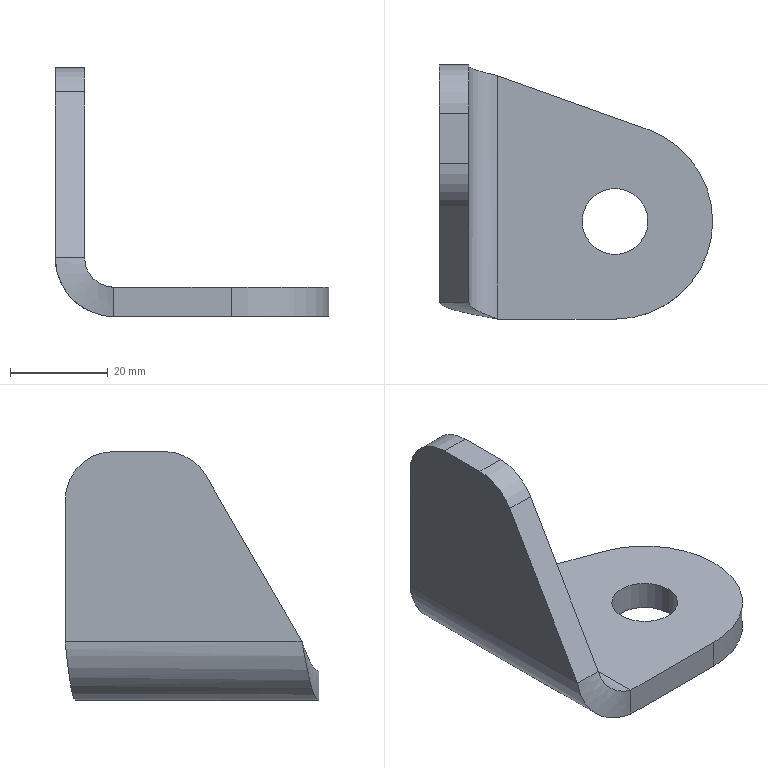Part | STEP file | Microwave Drying Flat Conveyor-CN2500x400-102-101 | 1 solid | 19 faces | box 56 x 52 x 51 mm | volume 22223 mm3 | plane 9 | cylinder 8 | spline 2 | commonest cylinder face diameters 13.489 x2 20 x2 40 x2 12 x1 24 x1
STEP:
#1=CARTESIAN_POINT('',(-6.745,0.,-6.));
#2=VERTEX_POINT('',#1);
#3=CARTESIAN_POINT('',(6.745,0.,-6.));
#4=VERTEX_POINT('',#3);
#5=CARTESIAN_POINT('',(0.,0.,-6.));
#6=DIRECTION('',(0.,0.,1.));
#7=DIRECTION('',(1.,0.,0.));
#8=AXIS2_PLACEMENT_3D('',#5,#6,#7);
#9=CIRCLE('',#8,6.745);
#10=EDGE_CURVE('',#2,#4,#9,.T.);
#11=ORIENTED_EDGE('',*,*,#10,.F.);
#12=CARTESIAN_POINT('',(-6.745,0.,0.));
#13=VERTEX_POINT('',#12);
#14=CARTESIAN_POINT('',(-6.745,0.,-6.));
#15=DIRECTION('',(0.,0.,1.));
#16=VECTOR('',#15,1000.);
#17=LINE('',#14,#16);
#18=EDGE_CURVE('',#2,#13,#17,.T.);
#19=ORIENTED_EDGE('',*,*,#18,.T.);
#20=CARTESIAN_POINT('',(6.745,0.,0.));
#21=VERTEX_POINT('',#20);
#22=CARTESIAN_POINT('',(0.,0.,0.));
#23=DIRECTION('',(0.,0.,1.));
#24=DIRECTION('',(1.,0.,0.));
#25=AXIS2_PLACEMENT_3D('',#22,#23,#24);
#26=CIRCLE('',#25,6.745);
#27=EDGE_CURVE('',#13,#21,#26,.T.);
#28=ORIENTED_EDGE('',*,*,#27,.T.);
#29=CARTESIAN_POINT('',(6.745,0.,-6.));
#30=DIRECTION('',(0.,0.,1.));
#31=VECTOR('',#30,1000.);
#32=LINE('',#29,#31);
#33=EDGE_CURVE('',#4,#21,#32,.T.);
#34=ORIENTED_EDGE('',*,*,#33,.F.);
#35=EDGE_LOOP('',(#11,#19,#28,#34));
#36=FACE_OUTER_BOUND('',#35,.T.);
#37=CARTESIAN_POINT('',(0.,0.,-6.));
#38=DIRECTION('',(0.,0.,1.));
#39=DIRECTION('',(1.,0.,0.));
#40=AXIS2_PLACEMENT_3D('',#37,#38,#39);
#41=CYLINDRICAL_SURFACE('',#40,6.745);
#42=ADVANCED_FACE('',(#36),#41,.F.);
#43=CARTESIAN_POINT('',(0.,-20.,-6.));
#44=VERTEX_POINT('',#43);
#45=CARTESIAN_POINT('',(20.,0.,-6.));
#46=VERTEX_POINT('',#45);
#47=CARTESIAN_POINT('',(0.,0.,-6.));
#48=DIRECTION('',(0.,0.,1.));
#49=DIRECTION('',(1.,0.,0.));
#50=AXIS2_PLACEMENT_3D('',#47,#48,#49);
#51=CIRCLE('',#50,20.);
#52=EDGE_CURVE('',#44,#46,#51,.T.);
#53=ORIENTED_EDGE('',*,*,#52,.T.);
#54=CARTESIAN_POINT('',(20.,0.,0.));
#55=VERTEX_POINT('',#54);
#56=CARTESIAN_POINT('',(20.,0.,-6.));
#57=DIRECTION('',(0.,0.,1.));
#58=VECTOR('',#57,1000.);
#59=LINE('',#56,#58);
#60=EDGE_CURVE('',#46,#55,#59,.T.);
#61=ORIENTED_EDGE('',*,*,#60,.T.);
#62=CARTESIAN_POINT('',(0.,-20.,0.));
#63=VERTEX_POINT('',#62);
#64=CARTESIAN_POINT('',(0.,0.,0.));
#65=DIRECTION('',(0.,0.,1.));
#66=DIRECTION('',(1.,0.,0.));
#67=AXIS2_PLACEMENT_3D('',#64,#65,#66);
#68=CIRCLE('',#67,20.);
#69=EDGE_CURVE('',#63,#55,#68,.T.);
#70=ORIENTED_EDGE('',*,*,#69,.F.);
#71=CARTESIAN_POINT('',(0.,-20.,-6.));
#72=DIRECTION('',(0.,0.,1.));
#73=VECTOR('',#72,1000.);
#74=LINE('',#71,#73);
#75=EDGE_CURVE('',#44,#63,#74,.T.);
#76=ORIENTED_EDGE('',*,*,#75,.F.);
#77=EDGE_LOOP('',(#53,#61,#70,#76));
#78=FACE_OUTER_BOUND('',#77,.T.);
#79=CARTESIAN_POINT('',(0.,0.,-6.));
#80=DIRECTION('',(0.,0.,1.));
#81=DIRECTION('',(1.,0.,0.));
#82=AXIS2_PLACEMENT_3D('',#79,#80,#81);
#83=CYLINDRICAL_SURFACE('',#82,20.);
#84=ADVANCED_FACE('',(#78),#83,.T.);
#85=CARTESIAN_POINT('',(-24.,-20.,0.));
#86=VERTEX_POINT('',#85);
#87=CARTESIAN_POINT('',(0.,-20.,0.));
#88=DIRECTION('',(1.,0.,0.));
#89=VECTOR('',#88,1000.);
#90=LINE('',#87,#89);
#91=EDGE_CURVE('',#86,#63,#90,.T.);
#92=ORIENTED_EDGE('',*,*,#91,.F.);
#93=CARTESIAN_POINT('',(-24.,-20.,-6.));
#94=VERTEX_POINT('',#93);
#95=CARTESIAN_POINT('',(-24.,-20.,0.));
#96=DIRECTION('',(0.,0.,-1.));
#97=VECTOR('',#96,1000.);
#98=LINE('',#95,#97);
#99=EDGE_CURVE('',#86,#94,#98,.T.);
#100=ORIENTED_EDGE('',*,*,#99,.T.);
#101=CARTESIAN_POINT('',(0.,-20.,-6.));
#102=DIRECTION('',(1.,0.,0.));
#103=VECTOR('',#102,1000.);
#104=LINE('',#101,#103);
#105=EDGE_CURVE('',#94,#44,#104,.T.);
#106=ORIENTED_EDGE('',*,*,#105,.T.);
#107=ORIENTED_EDGE('',*,*,#75,.T.);
#108=EDGE_LOOP('',(#92,#100,#106,#107));
#109=FACE_OUTER_BOUND('',#108,.T.);
#110=CARTESIAN_POINT('',(0.,-20.,-6.));
#111=DIRECTION('',(0.,-1.,0.));
#112=DIRECTION('',(1.,0.,0.));
#113=AXIS2_PLACEMENT_3D('',#110,#111,#112);
#114=PLANE('',#113);
#115=ADVANCED_FACE('',(#109),#114,.T.);
#116=CARTESIAN_POINT('',(0.,0.,-6.));
#117=DIRECTION('',(0.,0.,1.));
#118=DIRECTION('',(1.,0.,0.));
#119=AXIS2_PLACEMENT_3D('',#116,#117,#118);
#120=CIRCLE('',#119,6.745);
#121=EDGE_CURVE('',#4,#2,#120,.T.);
#122=ORIENTED_EDGE('',*,*,#121,.T.);
#123=ORIENTED_EDGE('',*,*,#10,.T.);
#124=EDGE_LOOP('',(#122,#123));
#125=FACE_BOUND('',#124,.T.);
#126=CARTESIAN_POINT('',(-24.,29.849,-6.));
#127=VERTEX_POINT('',#126);
#128=CARTESIAN_POINT('',(-24.,-20.,-6.));
#129=DIRECTION('',(0.,1.,0.));
#130=VECTOR('',#129,1000.);
#131=LINE('',#128,#130);
#132=EDGE_CURVE('',#94,#127,#131,.T.);
#133=ORIENTED_EDGE('',*,*,#132,.T.);
#134=CARTESIAN_POINT('',(6.749,18.827,-6.));
#135=VERTEX_POINT('',#134);
#136=CARTESIAN_POINT('',(6.749,18.827,-6.));
#137=DIRECTION('',(-0.9413,0.3374,0.));
#138=VECTOR('',#137,1000.);
#139=LINE('',#136,#138);
#140=EDGE_CURVE('',#135,#127,#139,.T.);
#141=ORIENTED_EDGE('',*,*,#140,.F.);
#142=CARTESIAN_POINT('',(0.,0.,-6.));
#143=DIRECTION('',(0.,0.,1.));
#144=DIRECTION('',(1.,0.,0.));
#145=AXIS2_PLACEMENT_3D('',#142,#143,#144);
#146=CIRCLE('',#145,20.);
#147=EDGE_CURVE('',#46,#135,#146,.T.);
#148=ORIENTED_EDGE('',*,*,#147,.F.);
#149=ORIENTED_EDGE('',*,*,#52,.F.);
#150=ORIENTED_EDGE('',*,*,#105,.F.);
#151=EDGE_LOOP('',(#133,#141,#148,#149,#150));
#152=FACE_OUTER_BOUND('',#151,.T.);
#153=CARTESIAN_POINT('',(0.,0.,-6.));
#154=DIRECTION('',(0.,0.,1.));
#155=DIRECTION('',(1.,0.,0.));
#156=AXIS2_PLACEMENT_3D('',#153,#154,#155);
#157=PLANE('',#156);
#158=ADVANCED_FACE('',(#125,#152),#157,.F.);
#159=CARTESIAN_POINT('',(0.,0.,0.));
#160=DIRECTION('',(0.,0.,1.));
#161=DIRECTION('',(1.,0.,0.));
#162=AXIS2_PLACEMENT_3D('',#159,#160,#161);
#163=CIRCLE('',#162,6.745);
#164=EDGE_CURVE('',#21,#13,#163,.T.);
#165=ORIENTED_EDGE('',*,*,#164,.F.);
#166=ORIENTED_EDGE('',*,*,#27,.F.);
#167=EDGE_LOOP('',(#165,#166));
#168=FACE_BOUND('',#167,.T.);
#169=CARTESIAN_POINT('',(6.749,18.827,0.));
#170=VERTEX_POINT('',#169);
#171=CARTESIAN_POINT('',(-24.,29.849,0.));
#172=VERTEX_POINT('',#171);
#173=CARTESIAN_POINT('',(6.749,18.827,0.));
#174=DIRECTION('',(-0.9413,0.3374,0.));
#175=VECTOR('',#174,1000.);
#176=LINE('',#173,#175);
#177=EDGE_CURVE('',#170,#172,#176,.T.);
#178=ORIENTED_EDGE('',*,*,#177,.T.);
#179=CARTESIAN_POINT('',(-24.,-20.,0.));
#180=DIRECTION('',(0.,1.,0.));
#181=VECTOR('',#180,1000.);
#182=LINE('',#179,#181);
#183=EDGE_CURVE('',#86,#172,#182,.T.);
#184=ORIENTED_EDGE('',*,*,#183,.F.);
#185=ORIENTED_EDGE('',*,*,#91,.T.);
#186=ORIENTED_EDGE('',*,*,#69,.T.);
#187=CARTESIAN_POINT('',(0.,0.,0.));
#188=DIRECTION('',(0.,0.,1.));
#189=DIRECTION('',(1.,0.,0.));
#190=AXIS2_PLACEMENT_3D('',#187,#188,#189);
#191=CIRCLE('',#190,20.);
#192=EDGE_CURVE('',#55,#170,#191,.T.);
#193=ORIENTED_EDGE('',*,*,#192,.T.);
#194=EDGE_LOOP('',(#178,#184,#185,#186,#193));
#195=FACE_OUTER_BOUND('',#194,.T.);
#196=CARTESIAN_POINT('',(0.,0.,0.));
#197=DIRECTION('',(0.,0.,1.));
#198=DIRECTION('',(1.,0.,0.));
#199=AXIS2_PLACEMENT_3D('',#196,#197,#198);
#200=PLANE('',#199);
#201=ADVANCED_FACE('',(#168,#195),#200,.T.);
#202=ORIENTED_EDGE('',*,*,#60,.F.);
#203=ORIENTED_EDGE('',*,*,#147,.T.);
#204=CARTESIAN_POINT('',(6.749,18.827,-6.));
#205=DIRECTION('',(0.,0.,1.));
#206=VECTOR('',#205,1000.);
#207=LINE('',#204,#206);
#208=EDGE_CURVE('',#135,#170,#207,.T.);
#209=ORIENTED_EDGE('',*,*,#208,.T.);
#210=ORIENTED_EDGE('',*,*,#192,.F.);
#211=EDGE_LOOP('',(#202,#203,#209,#210));
#212=FACE_OUTER_BOUND('',#211,.T.);
#213=CARTESIAN_POINT('',(0.,0.,-6.));
#214=DIRECTION('',(0.,0.,1.));
#215=DIRECTION('',(1.,0.,0.));
#216=AXIS2_PLACEMENT_3D('',#213,#214,#215);
#217=CYLINDRICAL_SURFACE('',#216,20.);
#218=ADVANCED_FACE('',(#212),#217,.T.);
#219=CARTESIAN_POINT('',(-24.,29.849,0.));
#220=DIRECTION('',(0.,0.,-1.));
#221=VECTOR('',#220,1000.);
#222=LINE('',#219,#221);
#223=EDGE_CURVE('',#172,#127,#222,.T.);
#224=ORIENTED_EDGE('',*,*,#223,.F.);
#225=ORIENTED_EDGE('',*,*,#177,.F.);
#226=ORIENTED_EDGE('',*,*,#208,.F.);
#227=ORIENTED_EDGE('',*,*,#140,.T.);
#228=EDGE_LOOP('',(#224,#225,#226,#227));
#229=FACE_OUTER_BOUND('',#228,.T.);
#230=CARTESIAN_POINT('',(6.749,18.827,-6.));
#231=DIRECTION('',(0.3374,0.9413,0.));
#232=DIRECTION('',(-0.9413,0.3374,0.));
#233=AXIS2_PLACEMENT_3D('',#230,#231,#232);
#234=PLANE('',#233);
#235=ADVANCED_FACE('',(#229),#234,.T.);
#236=ORIENTED_EDGE('',*,*,#18,.F.);
#237=ORIENTED_EDGE('',*,*,#121,.F.);
#238=ORIENTED_EDGE('',*,*,#33,.T.);
#239=ORIENTED_EDGE('',*,*,#164,.T.);
#240=EDGE_LOOP('',(#236,#237,#238,#239));
#241=FACE_OUTER_BOUND('',#240,.T.);
#242=CARTESIAN_POINT('',(0.,0.,-6.));
#243=DIRECTION('',(0.,0.,1.));
#244=DIRECTION('',(1.,0.,0.));
#245=AXIS2_PLACEMENT_3D('',#242,#243,#244);
#246=CYLINDRICAL_SURFACE('',#245,6.745);
#247=ADVANCED_FACE('',(#241),#246,.F.);
#248=CARTESIAN_POINT('',(-30.,32.,6.));
#249=VERTEX_POINT('',#248);
#250=CARTESIAN_POINT('',(-36.,32.,6.));
#251=VERTEX_POINT('',#250);
#252=CARTESIAN_POINT('',(-30.,32.,6.));
#253=DIRECTION('',(-1.,0.,0.));
#254=VECTOR('',#253,1000.);
#255=LINE('',#252,#254);
#256=EDGE_CURVE('',#249,#251,#255,.T.);
#257=ORIENTED_EDGE('',*,*,#256,.F.);
#258=CARTESIAN_POINT('',(-24.,29.849,0.));
#259=CARTESIAN_POINT('',(-24.396,29.94,0.));
#260=CARTESIAN_POINT('',(-24.786,30.029,0.03887));
#261=CARTESIAN_POINT('',(-25.361,30.162,0.153));
#262=CARTESIAN_POINT('',(-25.55,30.207,0.2005));
#263=CARTESIAN_POINT('',(-25.927,30.297,0.3144));
#264=CARTESIAN_POINT('',(-26.114,30.342,0.3814));
#265=CARTESIAN_POINT('',(-26.659,30.477,0.6072));
#266=CARTESIAN_POINT('',(-27.004,30.565,0.7915));
#267=CARTESIAN_POINT('',(-27.655,30.744,1.226));
#268=CARTESIAN_POINT('',(-27.964,30.835,1.479));
#269=CARTESIAN_POINT('',(-28.518,31.014,2.033));
#270=CARTESIAN_POINT('',(-28.766,31.102,2.335));
#271=CARTESIAN_POINT('',(-29.095,31.237,2.824));
#272=CARTESIAN_POINT('',(-29.197,31.282,2.995));
#273=CARTESIAN_POINT('',(-29.383,31.372,3.342));
#274=CARTESIAN_POINT('',(-29.467,31.417,3.519));
#275=CARTESIAN_POINT('',(-29.691,31.55,4.06));
#276=CARTESIAN_POINT('',(-29.806,31.639,4.435));
#277=CARTESIAN_POINT('',(-29.961,31.82,5.21));
#278=CARTESIAN_POINT('',(-30.,31.91,5.604));
#279=CARTESIAN_POINT('',(-30.,32.,6.));
#280=B_SPLINE_CURVE_WITH_KNOTS('',3,(#258,#259,#260,#261,#262,#263,#264,#265,#266,#267,#268,#269,#270,#271,#272,#273,#274,#275,#276,#277,#278,#279),.UNSPECIFIED.,.F.,.F.,(4,2,2,2,2,2,2,2,2,2,4),(0.,0.001202,0.001803,0.002403,0.003605,0.004807,0.006008,0.006609,0.00721,0.008412,0.009614),.UNSPECIFIED.);
#281=EDGE_CURVE('',#172,#249,#280,.T.);
#282=ORIENTED_EDGE('',*,*,#281,.F.);
#283=ORIENTED_EDGE('',*,*,#223,.T.);
#284=CARTESIAN_POINT('',(-24.,29.849,-6.));
#285=CARTESIAN_POINT('',(-24.792,29.94,-6.));
#286=CARTESIAN_POINT('',(-25.571,30.029,-5.922));
#287=CARTESIAN_POINT('',(-26.721,30.162,-5.694));
#288=CARTESIAN_POINT('',(-27.101,30.207,-5.599));
#289=CARTESIAN_POINT('',(-27.854,30.297,-5.371));
#290=CARTESIAN_POINT('',(-28.229,30.342,-5.237));
#291=CARTESIAN_POINT('',(-29.319,30.477,-4.786));
#292=CARTESIAN_POINT('',(-30.008,30.565,-4.417));
#293=CARTESIAN_POINT('',(-30.985,30.699,-3.765));
#294=CARTESIAN_POINT('',(-31.302,30.744,-3.531));
#295=CARTESIAN_POINT('',(-31.914,30.835,-3.029));
#296=CARTESIAN_POINT('',(-32.205,30.879,-2.765));
#297=CARTESIAN_POINT('',(-33.036,31.013,-1.935));
#298=CARTESIAN_POINT('',(-33.532,31.102,-1.332));
#299=CARTESIAN_POINT('',(-34.19,31.237,-0.3497));
#300=CARTESIAN_POINT('',(-34.395,31.282,-0.008866));
#301=CARTESIAN_POINT('',(-34.765,31.372,0.6838));
#302=CARTESIAN_POINT('',(-34.933,31.417,1.037));
#303=CARTESIAN_POINT('',(-35.232,31.506,1.759));
#304=CARTESIAN_POINT('',(-35.364,31.55,2.127));
#305=CARTESIAN_POINT('',(-35.593,31.64,2.877));
#306=CARTESIAN_POINT('',(-35.69,31.685,3.26));
#307=CARTESIAN_POINT('',(-35.922,31.82,4.424));
#308=CARTESIAN_POINT('',(-36.,31.91,5.208));
#309=CARTESIAN_POINT('',(-36.,32.,6.));
#310=B_SPLINE_CURVE_WITH_KNOTS('',3,(#284,#285,#286,#287,#288,#289,#290,#291,#292,#293,#294,#295,#296,#297,#298,#299,#300,#301,#302,#303,#304,#305,#306,#307,#308,#309),.UNSPECIFIED.,.F.,.F.,(4,2,2,2,2,2,2,2,2,2,2,2,4),(0.,0.002358,0.003538,0.004717,0.007075,0.008254,0.009434,0.01179,0.01297,0.01415,0.01533,0.01651,0.01887),.UNSPECIFIED.);
#311=EDGE_CURVE('',#127,#251,#310,.T.);
#312=ORIENTED_EDGE('',*,*,#311,.T.);
#313=EDGE_LOOP('',(#257,#282,#283,#312));
#314=FACE_OUTER_BOUND('',#313,.T.);
#315=CARTESIAN_POINT('',(-24.,29.849,-6.06));
#316=CARTESIAN_POINT('',(-25.579,30.028,-6.06));
#317=CARTESIAN_POINT('',(-27.157,30.208,-5.746));
#318=CARTESIAN_POINT('',(-30.074,30.566,-4.538));
#319=CARTESIAN_POINT('',(-31.411,30.745,-3.644));
#320=CARTESIAN_POINT('',(-33.644,31.104,-1.411));
#321=CARTESIAN_POINT('',(-34.538,31.283,-0.07364));
#322=CARTESIAN_POINT('',(-35.746,31.642,2.843));
#323=CARTESIAN_POINT('',(-36.06,31.821,4.421));
#324=CARTESIAN_POINT('',(-36.06,32.,6.));
#325=CARTESIAN_POINT('',(-24.,29.849,-6.));
#326=CARTESIAN_POINT('',(-25.571,30.028,-6.));
#327=CARTESIAN_POINT('',(-27.141,30.208,-5.688));
#328=CARTESIAN_POINT('',(-30.043,30.566,-4.485));
#329=CARTESIAN_POINT('',(-31.375,30.745,-3.596));
#330=CARTESIAN_POINT('',(-33.596,31.104,-1.375));
#331=CARTESIAN_POINT('',(-34.485,31.283,-0.04343));
#332=CARTESIAN_POINT('',(-35.688,31.642,2.859));
#333=CARTESIAN_POINT('',(-36.,31.821,4.429));
#334=CARTESIAN_POINT('',(-36.,32.,6.));
#335=CARTESIAN_POINT('',(-24.,29.849,0.));
#336=CARTESIAN_POINT('',(-24.786,30.028,0.));
#337=CARTESIAN_POINT('',(-25.57,30.208,0.1562));
#338=CARTESIAN_POINT('',(-27.022,30.566,0.7573));
#339=CARTESIAN_POINT('',(-27.687,30.745,1.202));
#340=CARTESIAN_POINT('',(-28.798,31.104,2.313));
#341=CARTESIAN_POINT('',(-29.243,31.283,2.978));
#342=CARTESIAN_POINT('',(-29.844,31.642,4.43));
#343=CARTESIAN_POINT('',(-30.,31.821,5.214));
#344=CARTESIAN_POINT('',(-30.,32.,6.));
#345=CARTESIAN_POINT('',(-24.,29.849,0.0606));
#346=CARTESIAN_POINT('',(-24.778,30.028,0.0606));
#347=CARTESIAN_POINT('',(-25.555,30.208,0.2152));
#348=CARTESIAN_POINT('',(-26.991,30.566,0.8102));
#349=CARTESIAN_POINT('',(-27.65,30.745,1.25));
#350=CARTESIAN_POINT('',(-28.75,31.104,2.35));
#351=CARTESIAN_POINT('',(-29.19,31.283,3.009));
#352=CARTESIAN_POINT('',(-29.785,31.642,4.445));
#353=CARTESIAN_POINT('',(-29.939,31.821,5.222));
#354=CARTESIAN_POINT('',(-29.939,32.,6.));
#355=B_SPLINE_SURFACE_WITH_KNOTS('',1,3,((#315,#316,#317,#318,#319,#320,#321,#322,#323,#324),(#325,#326,#327,#328,#329,#330,#331,#332,#333,#334),(#335,#336,#337,#338,#339,#340,#341,#342,#343,#344),(#345,#346,#347,#348,#349,#350,#351,#352,#353,#354)),.UNSPECIFIED.,.F.,.F.,.F.,(2,1,1,2),(4,2,2,2,4),(-0.01,0.,1.,1.01),(0.,0.25,0.5,0.75,1.),.UNSPECIFIED.);
#356=ADVANCED_FACE('',(#314),#355,.F.);
#357=CARTESIAN_POINT('',(-30.,-16.536,6.));
#358=VERTEX_POINT('',#357);
#359=CARTESIAN_POINT('',(-30.,-16.536,6.));
#360=CARTESIAN_POINT('',(-30.,-16.682,5.604));
#361=CARTESIAN_POINT('',(-29.961,-16.825,5.214));
#362=CARTESIAN_POINT('',(-29.847,-17.04,4.639));
#363=CARTESIAN_POINT('',(-29.799,-17.112,4.449));
#364=CARTESIAN_POINT('',(-29.686,-17.256,4.073));
#365=CARTESIAN_POINT('',(-29.619,-17.329,3.886));
#366=CARTESIAN_POINT('',(-29.392,-17.547,3.34));
#367=CARTESIAN_POINT('',(-29.208,-17.69,2.995));
#368=CARTESIAN_POINT('',(-28.882,-17.905,2.507));
#369=CARTESIAN_POINT('',(-28.766,-17.977,2.349));
#370=CARTESIAN_POINT('',(-28.516,-18.122,2.044));
#371=CARTESIAN_POINT('',(-28.382,-18.195,1.897));
#372=CARTESIAN_POINT('',(-27.966,-18.412,1.48));
#373=CARTESIAN_POINT('',(-27.664,-18.555,1.232));
#374=CARTESIAN_POINT('',(-27.013,-18.843,0.7965));
#375=CARTESIAN_POINT('',(-26.661,-18.989,0.608));
#376=CARTESIAN_POINT('',(-25.937,-19.277,0.3078));
#377=CARTESIAN_POINT('',(-25.563,-19.42,0.1939));
#378=CARTESIAN_POINT('',(-24.793,-19.709,0.03966));
#379=CARTESIAN_POINT('',(-24.396,-19.854,0.));
#380=CARTESIAN_POINT('',(-24.,-20.,0.));
#381=B_SPLINE_CURVE_WITH_KNOTS('',3,(#359,#360,#361,#362,#363,#364,#365,#366,#367,#368,#369,#370,#371,#372,#373,#374,#375,#376,#377,#378,#379,#380),.UNSPECIFIED.,.F.,.F.,(4,2,2,2,2,2,2,2,2,2,4),(0.,0.001248,0.001873,0.002497,0.003745,0.004369,0.004993,0.006242,0.00749,0.008738,0.009987),.UNSPECIFIED.);
#382=EDGE_CURVE('',#358,#86,#381,.T.);
#383=ORIENTED_EDGE('',*,*,#382,.F.);
#384=CARTESIAN_POINT('',(-36.,-16.536,6.));
#385=VERTEX_POINT('',#384);
#386=CARTESIAN_POINT('',(-30.,-16.536,6.));
#387=DIRECTION('',(-1.,0.,0.));
#388=VECTOR('',#387,1000.);
#389=LINE('',#386,#388);
#390=EDGE_CURVE('',#358,#385,#389,.T.);
#391=ORIENTED_EDGE('',*,*,#390,.T.);
#392=CARTESIAN_POINT('',(-36.,-16.536,6.));
#393=CARTESIAN_POINT('',(-36.,-16.682,5.208));
#394=CARTESIAN_POINT('',(-35.922,-16.825,4.428));
#395=CARTESIAN_POINT('',(-35.694,-17.04,3.279));
#396=CARTESIAN_POINT('',(-35.599,-17.112,2.899));
#397=CARTESIAN_POINT('',(-35.371,-17.257,2.146));
#398=CARTESIAN_POINT('',(-35.237,-17.33,1.772));
#399=CARTESIAN_POINT('',(-34.786,-17.546,0.6813));
#400=CARTESIAN_POINT('',(-34.417,-17.689,-0.007816));
#401=CARTESIAN_POINT('',(-33.548,-17.977,-1.311));
#402=CARTESIAN_POINT('',(-33.042,-18.123,-1.928));
#403=CARTESIAN_POINT('',(-31.935,-18.411,-3.036));
#404=CARTESIAN_POINT('',(-31.331,-18.554,-3.533));
#405=CARTESIAN_POINT('',(-30.351,-18.771,-4.189));
#406=CARTESIAN_POINT('',(-30.01,-18.844,-4.394));
#407=CARTESIAN_POINT('',(-29.316,-18.988,-4.765));
#408=CARTESIAN_POINT('',(-28.962,-19.06,-4.933));
#409=CARTESIAN_POINT('',(-27.88,-19.276,-5.382));
#410=CARTESIAN_POINT('',(-27.131,-19.419,-5.611));
#411=CARTESIAN_POINT('',(-25.577,-19.71,-5.922));
#412=CARTESIAN_POINT('',(-24.792,-19.854,-6.));
#413=CARTESIAN_POINT('',(-24.,-20.,-6.));
#414=B_SPLINE_CURVE_WITH_KNOTS('',3,(#392,#393,#394,#395,#396,#397,#398,#399,#400,#401,#402,#403,#404,#405,#406,#407,#408,#409,#410,#411,#412,#413),.UNSPECIFIED.,.F.,.F.,(4,2,2,2,2,2,2,2,2,2,4),(0.,0.002382,0.003574,0.004765,0.007147,0.00953,0.01191,0.0131,0.01429,0.01668,0.01906),.UNSPECIFIED.);
#415=EDGE_CURVE('',#385,#94,#414,.T.);
#416=ORIENTED_EDGE('',*,*,#415,.T.);
#417=ORIENTED_EDGE('',*,*,#99,.F.);
#418=EDGE_LOOP('',(#383,#391,#416,#417));
#419=FACE_OUTER_BOUND('',#418,.T.);
#420=CARTESIAN_POINT('',(-36.06,-16.536,6.));
#421=CARTESIAN_POINT('',(-36.06,-16.825,4.421));
#422=CARTESIAN_POINT('',(-35.746,-17.113,2.843));
#423=CARTESIAN_POINT('',(-34.538,-17.691,-0.07364));
#424=CARTESIAN_POINT('',(-33.644,-17.979,-1.411));
#425=CARTESIAN_POINT('',(-31.411,-18.557,-3.644));
#426=CARTESIAN_POINT('',(-30.074,-18.845,-4.538));
#427=CARTESIAN_POINT('',(-27.157,-19.423,-5.746));
#428=CARTESIAN_POINT('',(-25.579,-19.711,-6.06));
#429=CARTESIAN_POINT('',(-24.,-20.,-6.06));
#430=CARTESIAN_POINT('',(-36.,-16.536,6.));
#431=CARTESIAN_POINT('',(-36.,-16.825,4.429));
#432=CARTESIAN_POINT('',(-35.688,-17.113,2.859));
#433=CARTESIAN_POINT('',(-34.485,-17.691,-0.04343));
#434=CARTESIAN_POINT('',(-33.596,-17.979,-1.375));
#435=CARTESIAN_POINT('',(-31.375,-18.557,-3.596));
#436=CARTESIAN_POINT('',(-30.043,-18.845,-4.485));
#437=CARTESIAN_POINT('',(-27.141,-19.423,-5.688));
#438=CARTESIAN_POINT('',(-25.571,-19.711,-6.));
#439=CARTESIAN_POINT('',(-24.,-20.,-6.));
#440=CARTESIAN_POINT('',(-30.,-16.536,6.));
#441=CARTESIAN_POINT('',(-30.,-16.825,5.214));
#442=CARTESIAN_POINT('',(-29.844,-17.113,4.43));
#443=CARTESIAN_POINT('',(-29.243,-17.691,2.978));
#444=CARTESIAN_POINT('',(-28.798,-17.979,2.313));
#445=CARTESIAN_POINT('',(-27.687,-18.557,1.202));
#446=CARTESIAN_POINT('',(-27.022,-18.845,0.7573));
#447=CARTESIAN_POINT('',(-25.57,-19.423,0.1562));
#448=CARTESIAN_POINT('',(-24.786,-19.711,0.));
#449=CARTESIAN_POINT('',(-24.,-20.,0.));
#450=CARTESIAN_POINT('',(-29.939,-16.536,6.));
#451=CARTESIAN_POINT('',(-29.939,-16.825,5.222));
#452=CARTESIAN_POINT('',(-29.785,-17.113,4.445));
#453=CARTESIAN_POINT('',(-29.19,-17.691,3.009));
#454=CARTESIAN_POINT('',(-28.75,-17.979,2.35));
#455=CARTESIAN_POINT('',(-27.65,-18.557,1.25));
#456=CARTESIAN_POINT('',(-26.991,-18.845,0.8102));
#457=CARTESIAN_POINT('',(-25.555,-19.423,0.2152));
#458=CARTESIAN_POINT('',(-24.778,-19.711,0.0606));
#459=CARTESIAN_POINT('',(-24.,-20.,0.0606));
#460=B_SPLINE_SURFACE_WITH_KNOTS('',1,3,((#420,#421,#422,#423,#424,#425,#426,#427,#428,#429),(#430,#431,#432,#433,#434,#435,#436,#437,#438,#439),(#440,#441,#442,#443,#444,#445,#446,#447,#448,#449),(#450,#451,#452,#453,#454,#455,#456,#457,#458,#459)),.UNSPECIFIED.,.F.,.F.,.F.,(2,1,1,2),(4,2,2,2,4),(-0.01,0.,1.,1.01),(0.,0.25,0.5,0.75,1.),.UNSPECIFIED.);
#461=ADVANCED_FACE('',(#419),#460,.F.);
#462=ORIENTED_EDGE('',*,*,#132,.F.);
#463=ORIENTED_EDGE('',*,*,#415,.F.);
#464=CARTESIAN_POINT('',(-36.,22.,6.));
#465=DIRECTION('',(0.,1.,0.));
#466=VECTOR('',#465,1000.);
#467=LINE('',#464,#466);
#468=EDGE_CURVE('',#385,#251,#467,.T.);
#469=ORIENTED_EDGE('',*,*,#468,.T.);
#470=ORIENTED_EDGE('',*,*,#311,.F.);
#471=EDGE_LOOP('',(#462,#463,#469,#470));
#472=FACE_OUTER_BOUND('',#471,.T.);
#473=CARTESIAN_POINT('',(-24.,-20.,6.));
#474=DIRECTION('',(0.,-1.,0.));
#475=DIRECTION('',(-1.,0.,0.));
#476=AXIS2_PLACEMENT_3D('',#473,#474,#475);
#477=CYLINDRICAL_SURFACE('',#476,12.);
#478=ADVANCED_FACE('',(#472),#477,.T.);
#479=ORIENTED_EDGE('',*,*,#183,.T.);
#480=ORIENTED_EDGE('',*,*,#281,.T.);
#481=CARTESIAN_POINT('',(-30.,32.,6.));
#482=DIRECTION('',(0.,-1.,0.));
#483=VECTOR('',#482,1000.);
#484=LINE('',#481,#483);
#485=EDGE_CURVE('',#249,#358,#484,.T.);
#486=ORIENTED_EDGE('',*,*,#485,.T.);
#487=ORIENTED_EDGE('',*,*,#382,.T.);
#488=EDGE_LOOP('',(#479,#480,#486,#487));
#489=FACE_OUTER_BOUND('',#488,.T.);
#490=CARTESIAN_POINT('',(-24.,-20.,6.));
#491=DIRECTION('',(0.,-1.,0.));
#492=DIRECTION('',(-1.,0.,0.));
#493=AXIS2_PLACEMENT_3D('',#490,#491,#492);
#494=CYLINDRICAL_SURFACE('',#493,6.);
#495=ADVANCED_FACE('',(#489),#494,.F.);
#496=ORIENTED_EDGE('',*,*,#256,.T.);
#497=CARTESIAN_POINT('',(-36.,32.,35.));
#498=VERTEX_POINT('',#497);
#499=CARTESIAN_POINT('',(-36.,32.,0.));
#500=DIRECTION('',(0.,0.,-1.));
#501=VECTOR('',#500,1000.);
#502=LINE('',#499,#501);
#503=EDGE_CURVE('',#498,#251,#502,.T.);
#504=ORIENTED_EDGE('',*,*,#503,.F.);
#505=CARTESIAN_POINT('',(-30.,32.,35.));
#506=VERTEX_POINT('',#505);
#507=CARTESIAN_POINT('',(-36.,32.,35.));
#508=DIRECTION('',(1.,0.,0.));
#509=VECTOR('',#508,1000.);
#510=LINE('',#507,#509);
#511=EDGE_CURVE('',#498,#506,#510,.T.);
#512=ORIENTED_EDGE('',*,*,#511,.T.);
#513=CARTESIAN_POINT('',(-30.,32.,0.));
#514=DIRECTION('',(0.,0.,-1.));
#515=VECTOR('',#514,1000.);
#516=LINE('',#513,#515);
#517=EDGE_CURVE('',#506,#249,#516,.T.);
#518=ORIENTED_EDGE('',*,*,#517,.T.);
#519=EDGE_LOOP('',(#496,#504,#512,#518));
#520=FACE_OUTER_BOUND('',#519,.T.);
#521=CARTESIAN_POINT('',(-36.,32.,0.));
#522=DIRECTION('',(0.,-1.,0.));
#523=DIRECTION('',(1.,0.,0.));
#524=AXIS2_PLACEMENT_3D('',#521,#522,#523);
#525=PLANE('',#524);
#526=ADVANCED_FACE('',(#520),#525,.F.);
#527=ORIENTED_EDGE('',*,*,#390,.F.);
#528=CARTESIAN_POINT('',(-30.,3.094,40.));
#529=VERTEX_POINT('',#528);
#530=CARTESIAN_POINT('',(-30.,3.094,40.));
#531=DIRECTION('',(0.,0.5,0.866));
#532=VECTOR('',#531,1000.);
#533=LINE('',#530,#532);
#534=EDGE_CURVE('',#358,#529,#533,.T.);
#535=ORIENTED_EDGE('',*,*,#534,.T.);
#536=CARTESIAN_POINT('',(-36.,3.094,40.));
#537=VERTEX_POINT('',#536);
#538=CARTESIAN_POINT('',(-36.,3.094,40.));
#539=DIRECTION('',(1.,0.,0.));
#540=VECTOR('',#539,1000.);
#541=LINE('',#538,#540);
#542=EDGE_CURVE('',#537,#529,#541,.T.);
#543=ORIENTED_EDGE('',*,*,#542,.F.);
#544=CARTESIAN_POINT('',(-36.,3.094,40.));
#545=DIRECTION('',(0.,0.5,0.866));
#546=VECTOR('',#545,1000.);
#547=LINE('',#544,#546);
#548=EDGE_CURVE('',#385,#537,#547,.T.);
#549=ORIENTED_EDGE('',*,*,#548,.F.);
#550=EDGE_LOOP('',(#527,#535,#543,#549));
#551=FACE_OUTER_BOUND('',#550,.T.);
#552=CARTESIAN_POINT('',(-36.,3.094,40.));
#553=DIRECTION('',(0.,0.866,-0.5));
#554=DIRECTION('',(0.,0.5,0.866));
#555=AXIS2_PLACEMENT_3D('',#552,#553,#554);
#556=PLANE('',#555);
#557=ADVANCED_FACE('',(#551),#556,.F.);
#558=ORIENTED_EDGE('',*,*,#468,.F.);
#559=ORIENTED_EDGE('',*,*,#548,.T.);
#560=CARTESIAN_POINT('',(-36.,11.754,45.));
#561=VERTEX_POINT('',#560);
#562=CARTESIAN_POINT('',(-36.,11.754,35.));
#563=DIRECTION('',(-1.,0.,0.));
#564=DIRECTION('',(0.,0.,-1.));
#565=AXIS2_PLACEMENT_3D('',#562,#563,#564);
#566=CIRCLE('',#565,10.);
#567=EDGE_CURVE('',#537,#561,#566,.T.);
#568=ORIENTED_EDGE('',*,*,#567,.T.);
#569=CARTESIAN_POINT('',(-36.,22.,45.));
#570=VERTEX_POINT('',#569);
#571=CARTESIAN_POINT('',(-36.,22.,45.));
#572=DIRECTION('',(0.,1.,0.));
#573=VECTOR('',#572,1000.);
#574=LINE('',#571,#573);
#575=EDGE_CURVE('',#561,#570,#574,.T.);
#576=ORIENTED_EDGE('',*,*,#575,.T.);
#577=CARTESIAN_POINT('',(-36.,22.,35.));
#578=DIRECTION('',(-1.,0.,0.));
#579=DIRECTION('',(0.,0.,-1.));
#580=AXIS2_PLACEMENT_3D('',#577,#578,#579);
#581=CIRCLE('',#580,10.);
#582=EDGE_CURVE('',#570,#498,#581,.T.);
#583=ORIENTED_EDGE('',*,*,#582,.T.);
#584=ORIENTED_EDGE('',*,*,#503,.T.);
#585=EDGE_LOOP('',(#558,#559,#568,#576,#583,#584));
#586=FACE_OUTER_BOUND('',#585,.T.);
#587=CARTESIAN_POINT('',(-36.,22.,35.));
#588=DIRECTION('',(1.,0.,0.));
#589=DIRECTION('',(0.,0.,-1.));
#590=AXIS2_PLACEMENT_3D('',#587,#588,#589);
#591=PLANE('',#590);
#592=ADVANCED_FACE('',(#586),#591,.F.);
#593=ORIENTED_EDGE('',*,*,#534,.F.);
#594=ORIENTED_EDGE('',*,*,#485,.F.);
#595=ORIENTED_EDGE('',*,*,#517,.F.);
#596=CARTESIAN_POINT('',(-30.,22.,45.));
#597=VERTEX_POINT('',#596);
#598=CARTESIAN_POINT('',(-30.,22.,35.));
#599=DIRECTION('',(-1.,0.,0.));
#600=DIRECTION('',(0.,0.,-1.));
#601=AXIS2_PLACEMENT_3D('',#598,#599,#600);
#602=CIRCLE('',#601,10.);
#603=EDGE_CURVE('',#597,#506,#602,.T.);
#604=ORIENTED_EDGE('',*,*,#603,.F.);
#605=CARTESIAN_POINT('',(-30.,11.754,45.));
#606=VERTEX_POINT('',#605);
#607=CARTESIAN_POINT('',(-30.,22.,45.));
#608=DIRECTION('',(0.,1.,0.));
#609=VECTOR('',#608,1000.);
#610=LINE('',#607,#609);
#611=EDGE_CURVE('',#606,#597,#610,.T.);
#612=ORIENTED_EDGE('',*,*,#611,.F.);
#613=CARTESIAN_POINT('',(-30.,11.754,35.));
#614=DIRECTION('',(-1.,0.,0.));
#615=DIRECTION('',(0.,0.,-1.));
#616=AXIS2_PLACEMENT_3D('',#613,#614,#615);
#617=CIRCLE('',#616,10.);
#618=EDGE_CURVE('',#529,#606,#617,.T.);
#619=ORIENTED_EDGE('',*,*,#618,.F.);
#620=EDGE_LOOP('',(#593,#594,#595,#604,#612,#619));
#621=FACE_OUTER_BOUND('',#620,.T.);
#622=CARTESIAN_POINT('',(-30.,22.,35.));
#623=DIRECTION('',(1.,0.,0.));
#624=DIRECTION('',(0.,0.,-1.));
#625=AXIS2_PLACEMENT_3D('',#622,#623,#624);
#626=PLANE('',#625);
#627=ADVANCED_FACE('',(#621),#626,.T.);
#628=ORIENTED_EDGE('',*,*,#618,.T.);
#629=CARTESIAN_POINT('',(-36.,11.754,45.));
#630=DIRECTION('',(1.,0.,0.));
#631=VECTOR('',#630,1000.);
#632=LINE('',#629,#631);
#633=EDGE_CURVE('',#561,#606,#632,.T.);
#634=ORIENTED_EDGE('',*,*,#633,.F.);
#635=ORIENTED_EDGE('',*,*,#567,.F.);
#636=ORIENTED_EDGE('',*,*,#542,.T.);
#637=EDGE_LOOP('',(#628,#634,#635,#636));
#638=FACE_OUTER_BOUND('',#637,.T.);
#639=CARTESIAN_POINT('',(-36.,11.754,35.));
#640=DIRECTION('',(1.,0.,0.));
#641=DIRECTION('',(0.,0.,-1.));
#642=AXIS2_PLACEMENT_3D('',#639,#640,#641);
#643=CYLINDRICAL_SURFACE('',#642,10.);
#644=ADVANCED_FACE('',(#638),#643,.T.);
#645=ORIENTED_EDGE('',*,*,#611,.T.);
#646=CARTESIAN_POINT('',(-36.,22.,45.));
#647=DIRECTION('',(1.,0.,0.));
#648=VECTOR('',#647,1000.);
#649=LINE('',#646,#648);
#650=EDGE_CURVE('',#570,#597,#649,.T.);
#651=ORIENTED_EDGE('',*,*,#650,.F.);
#652=ORIENTED_EDGE('',*,*,#575,.F.);
#653=ORIENTED_EDGE('',*,*,#633,.T.);
#654=EDGE_LOOP('',(#645,#651,#652,#653));
#655=FACE_OUTER_BOUND('',#654,.T.);
#656=CARTESIAN_POINT('',(-36.,22.,45.));
#657=DIRECTION('',(0.,0.,-1.));
#658=DIRECTION('',(-1.,0.,0.));
#659=AXIS2_PLACEMENT_3D('',#656,#657,#658);
#660=PLANE('',#659);
#661=ADVANCED_FACE('',(#655),#660,.F.);
#662=ORIENTED_EDGE('',*,*,#603,.T.);
#663=ORIENTED_EDGE('',*,*,#511,.F.);
#664=ORIENTED_EDGE('',*,*,#582,.F.);
#665=ORIENTED_EDGE('',*,*,#650,.T.);
#666=EDGE_LOOP('',(#662,#663,#664,#665));
#667=FACE_OUTER_BOUND('',#666,.T.);
#668=CARTESIAN_POINT('',(-36.,22.,35.));
#669=DIRECTION('',(1.,0.,0.));
#670=DIRECTION('',(0.,0.,-1.));
#671=AXIS2_PLACEMENT_3D('',#668,#669,#670);
#672=CYLINDRICAL_SURFACE('',#671,10.);
#673=ADVANCED_FACE('',(#667),#672,.T.);
#674=CLOSED_SHELL('',(#42,#84,#115,#158,#201,#218,#235,#247,#356,#461,#478,#495,#526,#557,#592,#627,#644,#661,#673));
#675=MANIFOLD_SOLID_BREP('',#674);
#676=CARTESIAN_POINT('',(0.,0.,0.));
#677=DIRECTION('',(0.,0.,1.));
#678=DIRECTION('',(1.,0.,0.));
#679=AXIS2_PLACEMENT_3D('',#676,#677,#678);
#680=(LENGTH_UNIT()NAMED_UNIT(*)SI_UNIT(.MILLI.,.METRE.));
#681=UNCERTAINTY_MEASURE_WITH_UNIT(LENGTH_MEASURE(0.00001),#680,'','');
#682=(NAMED_UNIT(*)PLANE_ANGLE_UNIT()SI_UNIT($,.RADIAN.));
#683=(NAMED_UNIT(*)SI_UNIT($,.STERADIAN.)SOLID_ANGLE_UNIT());
#684=(GEOMETRIC_REPRESENTATION_CONTEXT(3)GLOBAL_UNCERTAINTY_ASSIGNED_CONTEXT((#681))GLOBAL_UNIT_ASSIGNED_CONTEXT((#680,#682,#683))REPRESENTATION_CONTEXT('',''));
#685=ADVANCED_BREP_SHAPE_REPRESENTATION('',(#675,#679),#684);